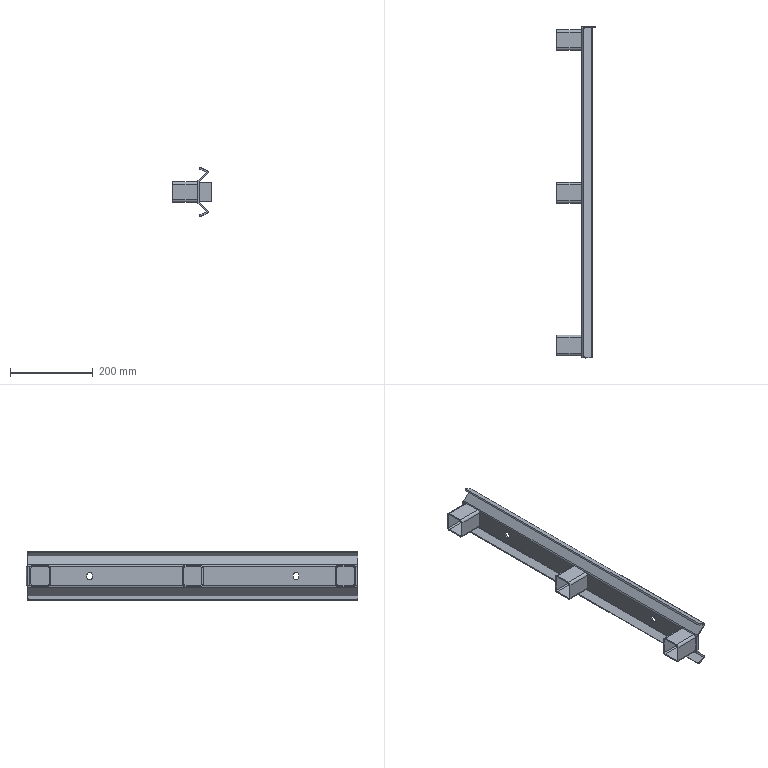Part | SolidWorks | 4 solids | 114 faces | box 94 x 804 x 120.238 mm | volume 609278 mm3 | plane 70 | cylinder 44 | commonest cylinder face diameters 6 x12 12 x12 10 x6 13 x6 0.2 x3 8.2 x3